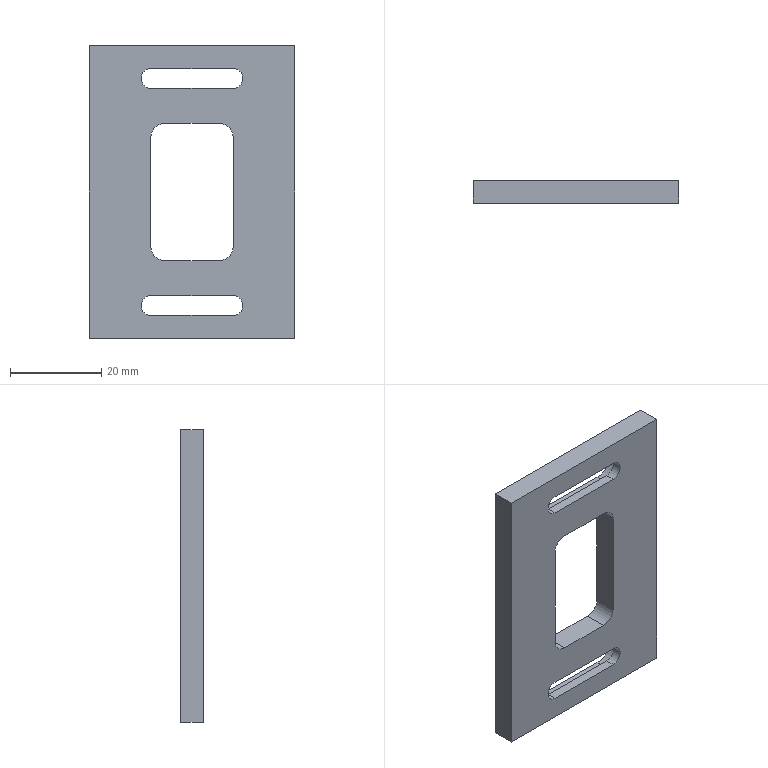Part | SolidWorks | features ICE 2, Extrusion 1, Fillet 1 | 1 solid | 32 faces | box 45 x 5 x 64 mm | volume 10150 mm3 | plane 20 | cylinder 12 | commonest cylinder face diameters 4.3 x4 6 x4 8.3 x4
STEP:
#1=CARTESIAN_POINT('',(-9.,5.,20.7));
#2=VERTEX_POINT('',#1);
#3=CARTESIAN_POINT('',(9.,5.,20.7));
#4=VERTEX_POINT('',#3);
#5=CARTESIAN_POINT('',(-9.,5.,20.7));
#6=DIRECTION('',(1.,0.,0.));
#7=VECTOR('',#6,1000.);
#8=LINE('',#5,#7);
#9=EDGE_CURVE('',#2,#4,#8,.T.);
#10=ORIENTED_EDGE('',*,*,#9,.T.);
#11=CARTESIAN_POINT('',(9.,5.,29.));
#12=VERTEX_POINT('',#11);
#13=CARTESIAN_POINT('',(9.,5.,24.85));
#14=DIRECTION('',(0.,1.,0.));
#15=DIRECTION('',(0.,0.,1.));
#16=AXIS2_PLACEMENT_3D('',#13,#14,#15);
#17=CIRCLE('',#16,4.15);
#18=EDGE_CURVE('',#12,#4,#17,.T.);
#19=ORIENTED_EDGE('',*,*,#18,.F.);
#20=CARTESIAN_POINT('',(-9.,5.,29.));
#21=VERTEX_POINT('',#20);
#22=CARTESIAN_POINT('',(-9.,5.,29.));
#23=DIRECTION('',(1.,0.,0.));
#24=VECTOR('',#23,1000.);
#25=LINE('',#22,#24);
#26=EDGE_CURVE('',#21,#12,#25,.T.);
#27=ORIENTED_EDGE('',*,*,#26,.F.);
#28=CARTESIAN_POINT('',(-9.,5.,24.85));
#29=DIRECTION('',(0.,1.,0.));
#30=DIRECTION('',(0.,0.,1.));
#31=AXIS2_PLACEMENT_3D('',#28,#29,#30);
#32=CIRCLE('',#31,4.15);
#33=EDGE_CURVE('',#2,#21,#32,.T.);
#34=ORIENTED_EDGE('',*,*,#33,.F.);
#35=EDGE_LOOP('',(#10,#19,#27,#34));
#36=FACE_BOUND('',#35,.T.);
#37=CARTESIAN_POINT('',(22.5,5.,32.));
#38=VERTEX_POINT('',#37);
#39=CARTESIAN_POINT('',(22.5,5.,-32.));
#40=VERTEX_POINT('',#39);
#41=CARTESIAN_POINT('',(22.5,5.,32.));
#42=DIRECTION('',(0.,0.,-1.));
#43=VECTOR('',#42,1000.);
#44=LINE('',#41,#43);
#45=EDGE_CURVE('',#38,#40,#44,.T.);
#46=ORIENTED_EDGE('',*,*,#45,.T.);
#47=CARTESIAN_POINT('',(-22.5,5.,-32.));
#48=VERTEX_POINT('',#47);
#49=CARTESIAN_POINT('',(-22.5,5.,-32.));
#50=DIRECTION('',(-1.,0.,0.));
#51=VECTOR('',#50,1000.);
#52=LINE('',#49,#51);
#53=EDGE_CURVE('',#40,#48,#52,.T.);
#54=ORIENTED_EDGE('',*,*,#53,.T.);
#55=CARTESIAN_POINT('',(-22.5,5.,32.));
#56=VERTEX_POINT('',#55);
#57=CARTESIAN_POINT('',(-22.5,5.,32.));
#58=DIRECTION('',(0.,0.,1.));
#59=VECTOR('',#58,1000.);
#60=LINE('',#57,#59);
#61=EDGE_CURVE('',#48,#56,#60,.T.);
#62=ORIENTED_EDGE('',*,*,#61,.T.);
#63=CARTESIAN_POINT('',(-22.5,5.,32.));
#64=DIRECTION('',(1.,0.,0.));
#65=VECTOR('',#64,1000.);
#66=LINE('',#63,#65);
#67=EDGE_CURVE('',#56,#38,#66,.T.);
#68=ORIENTED_EDGE('',*,*,#67,.T.);
#69=EDGE_LOOP('',(#46,#54,#62,#68));
#70=FACE_OUTER_BOUND('',#69,.T.);
#71=CARTESIAN_POINT('',(-9.,5.,12.));
#72=VERTEX_POINT('',#71);
#73=CARTESIAN_POINT('',(-9.,5.,-12.));
#74=VERTEX_POINT('',#73);
#75=CARTESIAN_POINT('',(-9.,5.,15.));
#76=DIRECTION('',(0.,0.,-1.));
#77=VECTOR('',#76,1000.);
#78=LINE('',#75,#77);
#79=EDGE_CURVE('',#72,#74,#78,.T.);
#80=ORIENTED_EDGE('',*,*,#79,.T.);
#81=CARTESIAN_POINT('',(-6.,5.,-15.));
#82=VERTEX_POINT('',#81);
#83=CARTESIAN_POINT('',(-6.,5.,-12.));
#84=DIRECTION('',(0.,-1.,0.));
#85=DIRECTION('',(0.,0.,-1.));
#86=AXIS2_PLACEMENT_3D('',#83,#84,#85);
#87=CIRCLE('',#86,3.);
#88=EDGE_CURVE('',#74,#82,#87,.T.);
#89=ORIENTED_EDGE('',*,*,#88,.T.);
#90=CARTESIAN_POINT('',(6.,5.,-15.));
#91=VERTEX_POINT('',#90);
#92=CARTESIAN_POINT('',(-9.,5.,-15.));
#93=DIRECTION('',(1.,0.,0.));
#94=VECTOR('',#93,1000.);
#95=LINE('',#92,#94);
#96=EDGE_CURVE('',#82,#91,#95,.T.);
#97=ORIENTED_EDGE('',*,*,#96,.T.);
#98=CARTESIAN_POINT('',(9.,5.,-12.));
#99=VERTEX_POINT('',#98);
#100=CARTESIAN_POINT('',(6.,5.,-12.));
#101=DIRECTION('',(0.,-1.,0.));
#102=DIRECTION('',(0.,0.,-1.));
#103=AXIS2_PLACEMENT_3D('',#100,#101,#102);
#104=CIRCLE('',#103,3.);
#105=EDGE_CURVE('',#91,#99,#104,.T.);
#106=ORIENTED_EDGE('',*,*,#105,.T.);
#107=CARTESIAN_POINT('',(9.,5.,12.));
#108=VERTEX_POINT('',#107);
#109=CARTESIAN_POINT('',(9.,5.,15.));
#110=DIRECTION('',(0.,0.,-1.));
#111=VECTOR('',#110,1000.);
#112=LINE('',#109,#111);
#113=EDGE_CURVE('',#108,#99,#112,.T.);
#114=ORIENTED_EDGE('',*,*,#113,.F.);
#115=CARTESIAN_POINT('',(6.,5.,15.));
#116=VERTEX_POINT('',#115);
#117=CARTESIAN_POINT('',(6.,5.,12.));
#118=DIRECTION('',(0.,-1.,0.));
#119=DIRECTION('',(0.,0.,-1.));
#120=AXIS2_PLACEMENT_3D('',#117,#118,#119);
#121=CIRCLE('',#120,3.);
#122=EDGE_CURVE('',#108,#116,#121,.T.);
#123=ORIENTED_EDGE('',*,*,#122,.T.);
#124=CARTESIAN_POINT('',(-6.,5.,15.));
#125=VERTEX_POINT('',#124);
#126=CARTESIAN_POINT('',(-9.,5.,15.));
#127=DIRECTION('',(1.,0.,0.));
#128=VECTOR('',#127,1000.);
#129=LINE('',#126,#128);
#130=EDGE_CURVE('',#125,#116,#129,.T.);
#131=ORIENTED_EDGE('',*,*,#130,.F.);
#132=CARTESIAN_POINT('',(-6.,5.,12.));
#133=DIRECTION('',(0.,-1.,0.));
#134=DIRECTION('',(0.,0.,-1.));
#135=AXIS2_PLACEMENT_3D('',#132,#133,#134);
#136=CIRCLE('',#135,3.);
#137=EDGE_CURVE('',#125,#72,#136,.T.);
#138=ORIENTED_EDGE('',*,*,#137,.T.);
#139=EDGE_LOOP('',(#80,#89,#97,#106,#114,#123,#131,#138));
#140=FACE_BOUND('',#139,.T.);
#141=CARTESIAN_POINT('',(9.,5.,-29.));
#142=VERTEX_POINT('',#141);
#143=CARTESIAN_POINT('',(9.,5.,-20.7));
#144=VERTEX_POINT('',#143);
#145=CARTESIAN_POINT('',(9.,5.,-24.85));
#146=DIRECTION('',(0.,-1.,0.));
#147=DIRECTION('',(0.,0.,-1.));
#148=AXIS2_PLACEMENT_3D('',#145,#146,#147);
#149=CIRCLE('',#148,4.15);
#150=EDGE_CURVE('',#142,#144,#149,.T.);
#151=ORIENTED_EDGE('',*,*,#150,.T.);
#152=CARTESIAN_POINT('',(-9.,5.,-20.7));
#153=VERTEX_POINT('',#152);
#154=CARTESIAN_POINT('',(-9.,5.,-20.7));
#155=DIRECTION('',(1.,0.,0.));
#156=VECTOR('',#155,1000.);
#157=LINE('',#154,#156);
#158=EDGE_CURVE('',#153,#144,#157,.T.);
#159=ORIENTED_EDGE('',*,*,#158,.F.);
#160=CARTESIAN_POINT('',(-9.,5.,-29.));
#161=VERTEX_POINT('',#160);
#162=CARTESIAN_POINT('',(-9.,5.,-24.85));
#163=DIRECTION('',(0.,-1.,0.));
#164=DIRECTION('',(0.,0.,-1.));
#165=AXIS2_PLACEMENT_3D('',#162,#163,#164);
#166=CIRCLE('',#165,4.15);
#167=EDGE_CURVE('',#153,#161,#166,.T.);
#168=ORIENTED_EDGE('',*,*,#167,.T.);
#169=CARTESIAN_POINT('',(-9.,5.,-29.));
#170=DIRECTION('',(1.,0.,0.));
#171=VECTOR('',#170,1000.);
#172=LINE('',#169,#171);
#173=EDGE_CURVE('',#161,#142,#172,.T.);
#174=ORIENTED_EDGE('',*,*,#173,.T.);
#175=EDGE_LOOP('',(#151,#159,#168,#174));
#176=FACE_BOUND('',#175,.T.);
#177=CARTESIAN_POINT('',(0.,5.,0.));
#178=DIRECTION('',(0.,-1.,0.));
#179=DIRECTION('',(0.,0.,-1.));
#180=AXIS2_PLACEMENT_3D('',#177,#178,#179);
#181=PLANE('',#180);
#182=ADVANCED_FACE('',(#36,#70,#140,#176),#181,.F.);
#183=CARTESIAN_POINT('',(-9.,2.,27.));
#184=VERTEX_POINT('',#183);
#185=CARTESIAN_POINT('',(-9.,2.,22.7));
#186=VERTEX_POINT('',#185);
#187=CARTESIAN_POINT('',(-9.,2.,24.85));
#188=DIRECTION('',(0.,-1.,0.));
#189=DIRECTION('',(0.,0.,1.));
#190=AXIS2_PLACEMENT_3D('',#187,#188,#189);
#191=CIRCLE('',#190,2.15);
#192=EDGE_CURVE('',#184,#186,#191,.T.);
#193=ORIENTED_EDGE('',*,*,#192,.F.);
#194=CARTESIAN_POINT('',(-9.,0.,27.));
#195=VERTEX_POINT('',#194);
#196=CARTESIAN_POINT('',(-9.,0.,27.));
#197=DIRECTION('',(0.,1.,0.));
#198=VECTOR('',#197,1000.);
#199=LINE('',#196,#198);
#200=EDGE_CURVE('',#195,#184,#199,.T.);
#201=ORIENTED_EDGE('',*,*,#200,.F.);
#202=CARTESIAN_POINT('',(-9.,0.,22.7));
#203=VERTEX_POINT('',#202);
#204=CARTESIAN_POINT('',(-9.,0.,24.85));
#205=DIRECTION('',(0.,1.,0.));
#206=DIRECTION('',(0.,0.,1.));
#207=AXIS2_PLACEMENT_3D('',#204,#205,#206);
#208=CIRCLE('',#207,2.15);
#209=EDGE_CURVE('',#203,#195,#208,.T.);
#210=ORIENTED_EDGE('',*,*,#209,.F.);
#211=CARTESIAN_POINT('',(-9.,0.,22.7));
#212=DIRECTION('',(0.,1.,0.));
#213=VECTOR('',#212,1000.);
#214=LINE('',#211,#213);
#215=EDGE_CURVE('',#203,#186,#214,.T.);
#216=ORIENTED_EDGE('',*,*,#215,.T.);
#217=EDGE_LOOP('',(#193,#201,#210,#216));
#218=FACE_OUTER_BOUND('',#217,.T.);
#219=CARTESIAN_POINT('',(-9.,0.,24.85));
#220=DIRECTION('',(0.,1.,0.));
#221=DIRECTION('',(0.,0.,1.));
#222=AXIS2_PLACEMENT_3D('',#219,#220,#221);
#223=CYLINDRICAL_SURFACE('',#222,2.15);
#224=ADVANCED_FACE('',(#218),#223,.F.);
#225=CARTESIAN_POINT('',(9.,0.,22.7));
#226=VERTEX_POINT('',#225);
#227=CARTESIAN_POINT('',(9.,2.,22.7));
#228=VERTEX_POINT('',#227);
#229=CARTESIAN_POINT('',(9.,0.,22.7));
#230=DIRECTION('',(0.,1.,0.));
#231=VECTOR('',#230,1000.);
#232=LINE('',#229,#231);
#233=EDGE_CURVE('',#226,#228,#232,.T.);
#234=ORIENTED_EDGE('',*,*,#233,.T.);
#235=CARTESIAN_POINT('',(-9.,2.,22.7));
#236=DIRECTION('',(-1.,0.,0.));
#237=VECTOR('',#236,1000.);
#238=LINE('',#235,#237);
#239=EDGE_CURVE('',#228,#186,#238,.T.);
#240=ORIENTED_EDGE('',*,*,#239,.T.);
#241=ORIENTED_EDGE('',*,*,#215,.F.);
#242=CARTESIAN_POINT('',(-9.,0.,22.7));
#243=DIRECTION('',(1.,0.,0.));
#244=VECTOR('',#243,1000.);
#245=LINE('',#242,#244);
#246=EDGE_CURVE('',#203,#226,#245,.T.);
#247=ORIENTED_EDGE('',*,*,#246,.T.);
#248=EDGE_LOOP('',(#234,#240,#241,#247));
#249=FACE_OUTER_BOUND('',#248,.T.);
#250=CARTESIAN_POINT('',(-9.,0.,22.7));
#251=DIRECTION('',(0.,0.,1.));
#252=DIRECTION('',(1.,0.,0.));
#253=AXIS2_PLACEMENT_3D('',#250,#251,#252);
#254=PLANE('',#253);
#255=ADVANCED_FACE('',(#249),#254,.T.);
#256=CARTESIAN_POINT('',(9.,2.,27.));
#257=VERTEX_POINT('',#256);
#258=CARTESIAN_POINT('',(9.,2.,24.85));
#259=DIRECTION('',(0.,-1.,0.));
#260=DIRECTION('',(0.,0.,1.));
#261=AXIS2_PLACEMENT_3D('',#258,#259,#260);
#262=CIRCLE('',#261,2.15);
#263=EDGE_CURVE('',#228,#257,#262,.T.);
#264=ORIENTED_EDGE('',*,*,#263,.F.);
#265=ORIENTED_EDGE('',*,*,#233,.F.);
#266=CARTESIAN_POINT('',(9.,0.,27.));
#267=VERTEX_POINT('',#266);
#268=CARTESIAN_POINT('',(9.,0.,24.85));
#269=DIRECTION('',(0.,1.,0.));
#270=DIRECTION('',(0.,0.,1.));
#271=AXIS2_PLACEMENT_3D('',#268,#269,#270);
#272=CIRCLE('',#271,2.15);
#273=EDGE_CURVE('',#267,#226,#272,.T.);
#274=ORIENTED_EDGE('',*,*,#273,.F.);
#275=CARTESIAN_POINT('',(9.,0.,27.));
#276=DIRECTION('',(0.,1.,0.));
#277=VECTOR('',#276,1000.);
#278=LINE('',#275,#277);
#279=EDGE_CURVE('',#267,#257,#278,.T.);
#280=ORIENTED_EDGE('',*,*,#279,.T.);
#281=EDGE_LOOP('',(#264,#265,#274,#280));
#282=FACE_OUTER_BOUND('',#281,.T.);
#283=CARTESIAN_POINT('',(9.,0.,24.85));
#284=DIRECTION('',(0.,1.,0.));
#285=DIRECTION('',(0.,0.,1.));
#286=AXIS2_PLACEMENT_3D('',#283,#284,#285);
#287=CYLINDRICAL_SURFACE('',#286,2.15);
#288=ADVANCED_FACE('',(#282),#287,.F.);
#289=CARTESIAN_POINT('',(-9.,2.,27.));
#290=DIRECTION('',(-1.,0.,0.));
#291=VECTOR('',#290,1000.);
#292=LINE('',#289,#291);
#293=EDGE_CURVE('',#257,#184,#292,.T.);
#294=ORIENTED_EDGE('',*,*,#293,.F.);
#295=ORIENTED_EDGE('',*,*,#279,.F.);
#296=CARTESIAN_POINT('',(-9.,0.,27.));
#297=DIRECTION('',(1.,0.,0.));
#298=VECTOR('',#297,1000.);
#299=LINE('',#296,#298);
#300=EDGE_CURVE('',#195,#267,#299,.T.);
#301=ORIENTED_EDGE('',*,*,#300,.F.);
#302=ORIENTED_EDGE('',*,*,#200,.T.);
#303=EDGE_LOOP('',(#294,#295,#301,#302));
#304=FACE_OUTER_BOUND('',#303,.T.);
#305=CARTESIAN_POINT('',(-9.,0.,27.));
#306=DIRECTION('',(0.,0.,1.));
#307=DIRECTION('',(1.,0.,0.));
#308=AXIS2_PLACEMENT_3D('',#305,#306,#307);
#309=PLANE('',#308);
#310=ADVANCED_FACE('',(#304),#309,.F.);
#311=ORIENTED_EDGE('',*,*,#209,.T.);
#312=ORIENTED_EDGE('',*,*,#300,.T.);
#313=ORIENTED_EDGE('',*,*,#273,.T.);
#314=ORIENTED_EDGE('',*,*,#246,.F.);
#315=EDGE_LOOP('',(#311,#312,#313,#314));
#316=FACE_BOUND('',#315,.T.);
#317=CARTESIAN_POINT('',(22.5,0.,32.));
#318=VERTEX_POINT('',#317);
#319=CARTESIAN_POINT('',(22.5,0.,-32.));
#320=VERTEX_POINT('',#319);
#321=CARTESIAN_POINT('',(22.5,0.,32.));
#322=DIRECTION('',(0.,0.,-1.));
#323=VECTOR('',#322,1000.);
#324=LINE('',#321,#323);
#325=EDGE_CURVE('',#318,#320,#324,.T.);
#326=ORIENTED_EDGE('',*,*,#325,.F.);
#327=CARTESIAN_POINT('',(-22.5,0.,32.));
#328=VERTEX_POINT('',#327);
#329=CARTESIAN_POINT('',(-22.5,0.,32.));
#330=DIRECTION('',(1.,0.,0.));
#331=VECTOR('',#330,1000.);
#332=LINE('',#329,#331);
#333=EDGE_CURVE('',#328,#318,#332,.T.);
#334=ORIENTED_EDGE('',*,*,#333,.F.);
#335=CARTESIAN_POINT('',(-22.5,0.,-32.));
#336=VERTEX_POINT('',#335);
#337=CARTESIAN_POINT('',(-22.5,0.,32.));
#338=DIRECTION('',(0.,0.,1.));
#339=VECTOR('',#338,1000.);
#340=LINE('',#337,#339);
#341=EDGE_CURVE('',#336,#328,#340,.T.);
#342=ORIENTED_EDGE('',*,*,#341,.F.);
#343=CARTESIAN_POINT('',(-22.5,0.,-32.));
#344=DIRECTION('',(-1.,0.,0.));
#345=VECTOR('',#344,1000.);
#346=LINE('',#343,#345);
#347=EDGE_CURVE('',#320,#336,#346,.T.);
#348=ORIENTED_EDGE('',*,*,#347,.F.);
#349=EDGE_LOOP('',(#326,#334,#342,#348));
#350=FACE_OUTER_BOUND('',#349,.T.);
#351=CARTESIAN_POINT('',(-6.,0.,15.));
#352=VERTEX_POINT('',#351);
#353=CARTESIAN_POINT('',(6.,0.,15.));
#354=VERTEX_POINT('',#353);
#355=CARTESIAN_POINT('',(-9.,0.,15.));
#356=DIRECTION('',(1.,0.,0.));
#357=VECTOR('',#356,1000.);
#358=LINE('',#355,#357);
#359=EDGE_CURVE('',#352,#354,#358,.T.);
#360=ORIENTED_EDGE('',*,*,#359,.T.);
#361=CARTESIAN_POINT('',(9.,0.,12.));
#362=VERTEX_POINT('',#361);
#363=CARTESIAN_POINT('',(6.,0.,12.));
#364=DIRECTION('',(0.,1.,0.));
#365=DIRECTION('',(0.,0.,-1.));
#366=AXIS2_PLACEMENT_3D('',#363,#364,#365);
#367=CIRCLE('',#366,3.);
#368=EDGE_CURVE('',#354,#362,#367,.T.);
#369=ORIENTED_EDGE('',*,*,#368,.T.);
#370=CARTESIAN_POINT('',(9.,0.,-12.));
#371=VERTEX_POINT('',#370);
#372=CARTESIAN_POINT('',(9.,0.,15.));
#373=DIRECTION('',(0.,0.,-1.));
#374=VECTOR('',#373,1000.);
#375=LINE('',#372,#374);
#376=EDGE_CURVE('',#362,#371,#375,.T.);
#377=ORIENTED_EDGE('',*,*,#376,.T.);
#378=CARTESIAN_POINT('',(6.,0.,-15.));
#379=VERTEX_POINT('',#378);
#380=CARTESIAN_POINT('',(6.,0.,-12.));
#381=DIRECTION('',(0.,1.,0.));
#382=DIRECTION('',(0.,0.,-1.));
#383=AXIS2_PLACEMENT_3D('',#380,#381,#382);
#384=CIRCLE('',#383,3.);
#385=EDGE_CURVE('',#371,#379,#384,.T.);
#386=ORIENTED_EDGE('',*,*,#385,.T.);
#387=CARTESIAN_POINT('',(-6.,0.,-15.));
#388=VERTEX_POINT('',#387);
#389=CARTESIAN_POINT('',(-9.,0.,-15.));
#390=DIRECTION('',(1.,0.,0.));
#391=VECTOR('',#390,1000.);
#392=LINE('',#389,#391);
#393=EDGE_CURVE('',#388,#379,#392,.T.);
#394=ORIENTED_EDGE('',*,*,#393,.F.);
#395=CARTESIAN_POINT('',(-9.,0.,-12.));
#396=VERTEX_POINT('',#395);
#397=CARTESIAN_POINT('',(-6.,0.,-12.));
#398=DIRECTION('',(0.,1.,0.));
#399=DIRECTION('',(0.,0.,-1.));
#400=AXIS2_PLACEMENT_3D('',#397,#398,#399);
#401=CIRCLE('',#400,3.);
#402=EDGE_CURVE('',#388,#396,#401,.T.);
#403=ORIENTED_EDGE('',*,*,#402,.T.);
#404=CARTESIAN_POINT('',(-9.,0.,12.));
#405=VERTEX_POINT('',#404);
#406=CARTESIAN_POINT('',(-9.,0.,15.));
#407=DIRECTION('',(0.,0.,-1.));
#408=VECTOR('',#407,1000.);
#409=LINE('',#406,#408);
#410=EDGE_CURVE('',#405,#396,#409,.T.);
#411=ORIENTED_EDGE('',*,*,#410,.F.);
#412=CARTESIAN_POINT('',(-6.,0.,12.));
#413=DIRECTION('',(0.,1.,0.));
#414=DIRECTION('',(0.,0.,-1.));
#415=AXIS2_PLACEMENT_3D('',#412,#413,#414);
#416=CIRCLE('',#415,3.);
#417=EDGE_CURVE('',#405,#352,#416,.T.);
#418=ORIENTED_EDGE('',*,*,#417,.T.);
#419=EDGE_LOOP('',(#360,#369,#377,#386,#394,#403,#411,#418));
#420=FACE_BOUND('',#419,.T.);
#421=CARTESIAN_POINT('',(-9.,0.,-27.));
#422=VERTEX_POINT('',#421);
#423=CARTESIAN_POINT('',(9.,0.,-27.));
#424=VERTEX_POINT('',#423);
#425=CARTESIAN_POINT('',(-9.,0.,-27.));
#426=DIRECTION('',(1.,0.,0.));
#427=VECTOR('',#426,1000.);
#428=LINE('',#425,#427);
#429=EDGE_CURVE('',#422,#424,#428,.T.);
#430=ORIENTED_EDGE('',*,*,#429,.F.);
#431=CARTESIAN_POINT('',(-9.,0.,-22.7));
#432=VERTEX_POINT('',#431);
#433=CARTESIAN_POINT('',(-9.,0.,-24.85));
#434=DIRECTION('',(0.,-1.,0.));
#435=DIRECTION('',(0.,0.,-1.));
#436=AXIS2_PLACEMENT_3D('',#433,#434,#435);
#437=CIRCLE('',#436,2.15);
#438=EDGE_CURVE('',#432,#422,#437,.T.);
#439=ORIENTED_EDGE('',*,*,#438,.F.);
#440=CARTESIAN_POINT('',(9.,0.,-22.7));
#441=VERTEX_POINT('',#440);
#442=CARTESIAN_POINT('',(-9.,0.,-22.7));
#443=DIRECTION('',(1.,0.,0.));
#444=VECTOR('',#443,1000.);
#445=LINE('',#442,#444);
#446=EDGE_CURVE('',#432,#441,#445,.T.);
#447=ORIENTED_EDGE('',*,*,#446,.T.);
#448=CARTESIAN_POINT('',(9.,0.,-24.85));
#449=DIRECTION('',(0.,-1.,0.));
#450=DIRECTION('',(0.,0.,-1.));
#451=AXIS2_PLACEMENT_3D('',#448,#449,#450);
#452=CIRCLE('',#451,2.15);
#453=EDGE_CURVE('',#424,#441,#452,.T.);
#454=ORIENTED_EDGE('',*,*,#453,.F.);
#455=EDGE_LOOP('',(#430,#439,#447,#454));
#456=FACE_BOUND('',#455,.T.);
#457=CARTESIAN_POINT('',(0.,0.,0.));
#458=DIRECTION('',(0.,-1.,0.));
#459=DIRECTION('',(0.,0.,-1.));
#460=AXIS2_PLACEMENT_3D('',#457,#458,#459);
#461=PLANE('',#460);
#462=ADVANCED_FACE('',(#316,#350,#420,#456),#461,.T.);
#463=ORIENTED_EDGE('',*,*,#325,.T.);
#464=CARTESIAN_POINT('',(22.5,5.,-32.));
#465=DIRECTION('',(0.,-1.,0.));
#466=VECTOR('',#465,1000.);
#467=LINE('',#464,#466);
#468=EDGE_CURVE('',#40,#320,#467,.T.);
#469=ORIENTED_EDGE('',*,*,#468,.F.);
#470=ORIENTED_EDGE('',*,*,#45,.F.);
#471=CARTESIAN_POINT('',(22.5,5.,32.));
#472=DIRECTION('',(0.,-1.,0.));
#473=VECTOR('',#472,1000.);
#474=LINE('',#471,#473);
#475=EDGE_CURVE('',#38,#318,#474,.T.);
#476=ORIENTED_EDGE('',*,*,#475,.T.);
#477=EDGE_LOOP('',(#463,#469,#470,#476));
#478=FACE_OUTER_BOUND('',#477,.T.);
#479=CARTESIAN_POINT('',(22.5,5.,32.));
#480=DIRECTION('',(-1.,0.,0.));
#481=DIRECTION('',(0.,0.,1.));
#482=AXIS2_PLACEMENT_3D('',#479,#480,#481);
#483=PLANE('',#482);
#484=ADVANCED_FACE('',(#478),#483,.F.);
#485=ORIENTED_EDGE('',*,*,#347,.T.);
#486=CARTESIAN_POINT('',(-22.5,5.,-32.));
#487=DIRECTION('',(0.,-1.,0.));
#488=VECTOR('',#487,1000.);
#489=LINE('',#486,#488);
#490=EDGE_CURVE('',#48,#336,#489,.T.);
#491=ORIENTED_EDGE('',*,*,#490,.F.);
#492=ORIENTED_EDGE('',*,*,#53,.F.);
#493=ORIENTED_EDGE('',*,*,#468,.T.);
#494=EDGE_LOOP('',(#485,#491,#492,#493));
#495=FACE_OUTER_BOUND('',#494,.T.);
#496=CARTESIAN_POINT('',(-22.5,5.,-32.));
#497=DIRECTION('',(0.,0.,1.));
#498=DIRECTION('',(1.,0.,0.));
#499=AXIS2_PLACEMENT_3D('',#496,#497,#498);
#500=PLANE('',#499);
#501=ADVANCED_FACE('',(#495),#500,.F.);
#502=ORIENTED_EDGE('',*,*,#341,.T.);
#503=CARTESIAN_POINT('',(-22.5,5.,32.));
#504=DIRECTION('',(0.,-1.,0.));
#505=VECTOR('',#504,1000.);
#506=LINE('',#503,#505);
#507=EDGE_CURVE('',#56,#328,#506,.T.);
#508=ORIENTED_EDGE('',*,*,#507,.F.);
#509=ORIENTED_EDGE('',*,*,#61,.F.);
#510=ORIENTED_EDGE('',*,*,#490,.T.);
#511=EDGE_LOOP('',(#502,#508,#509,#510));
#512=FACE_OUTER_BOUND('',#511,.T.);
#513=CARTESIAN_POINT('',(-22.5,5.,32.));
#514=DIRECTION('',(1.,0.,0.));
#515=DIRECTION('',(0.,0.,-1.));
#516=AXIS2_PLACEMENT_3D('',#513,#514,#515);
#517=PLANE('',#516);
#518=ADVANCED_FACE('',(#512),#517,.F.);
#519=ORIENTED_EDGE('',*,*,#333,.T.);
#520=ORIENTED_EDGE('',*,*,#475,.F.);
#521=ORIENTED_EDGE('',*,*,#67,.F.);
#522=ORIENTED_EDGE('',*,*,#507,.T.);
#523=EDGE_LOOP('',(#519,#520,#521,#522));
#524=FACE_OUTER_BOUND('',#523,.T.);
#525=CARTESIAN_POINT('',(-22.5,5.,32.));
#526=DIRECTION('',(0.,0.,-1.));
#527=DIRECTION('',(-1.,0.,0.));
#528=AXIS2_PLACEMENT_3D('',#525,#526,#527);
#529=PLANE('',#528);
#530=ADVANCED_FACE('',(#524),#529,.F.);
#531=ORIENTED_EDGE('',*,*,#393,.T.);
#532=CARTESIAN_POINT('',(6.,0.,-15.));
#533=DIRECTION('',(0.,1.,0.));
#534=VECTOR('',#533,1000.);
#535=LINE('',#532,#534);
#536=EDGE_CURVE('',#379,#91,#535,.T.);
#537=ORIENTED_EDGE('',*,*,#536,.T.);
#538=ORIENTED_EDGE('',*,*,#96,.F.);
#539=CARTESIAN_POINT('',(-6.,0.,-15.));
#540=DIRECTION('',(0.,-1.,0.));
#541=VECTOR('',#540,1000.);
#542=LINE('',#539,#541);
#543=EDGE_CURVE('',#82,#388,#542,.T.);
#544=ORIENTED_EDGE('',*,*,#543,.T.);
#545=EDGE_LOOP('',(#531,#537,#538,#544));
#546=FACE_OUTER_BOUND('',#545,.T.);
#547=CARTESIAN_POINT('',(-9.,0.,-15.));
#548=DIRECTION('',(0.,0.,1.));
#549=DIRECTION('',(1.,0.,0.));
#550=AXIS2_PLACEMENT_3D('',#547,#548,#549);
#551=PLANE('',#550);
#552=ADVANCED_FACE('',(#546),#551,.T.);
#553=ORIENTED_EDGE('',*,*,#113,.T.);
#554=CARTESIAN_POINT('',(9.,0.,-12.));
#555=DIRECTION('',(0.,-1.,0.));
#556=VECTOR('',#555,1000.);
#557=LINE('',#554,#556);
#558=EDGE_CURVE('',#99,#371,#557,.T.);
#559=ORIENTED_EDGE('',*,*,#558,.T.);
#560=ORIENTED_EDGE('',*,*,#376,.F.);
#561=CARTESIAN_POINT('',(9.,5.,12.));
#562=DIRECTION('',(0.,1.,0.));
#563=VECTOR('',#562,1000.);
#564=LINE('',#561,#563);
#565=EDGE_CURVE('',#362,#108,#564,.T.);
#566=ORIENTED_EDGE('',*,*,#565,.T.);
#567=EDGE_LOOP('',(#553,#559,#560,#566));
#568=FACE_OUTER_BOUND('',#567,.T.);
#569=CARTESIAN_POINT('',(9.,0.,15.));
#570=DIRECTION('',(1.,0.,0.));
#571=DIRECTION('',(0.,0.,-1.));
#572=AXIS2_PLACEMENT_3D('',#569,#570,#571);
#573=PLANE('',#572);
#574=ADVANCED_FACE('',(#568),#573,.F.);
#575=ORIENTED_EDGE('',*,*,#130,.T.);
#576=CARTESIAN_POINT('',(6.,0.,15.));
#577=DIRECTION('',(0.,-1.,0.));
#578=VECTOR('',#577,1000.);
#579=LINE('',#576,#578);
#580=EDGE_CURVE('',#116,#354,#579,.T.);
#581=ORIENTED_EDGE('',*,*,#580,.T.);
#582=ORIENTED_EDGE('',*,*,#359,.F.);
#583=CARTESIAN_POINT('',(-6.,0.,15.));
#584=DIRECTION('',(0.,1.,0.));
#585=VECTOR('',#584,1000.);
#586=LINE('',#583,#585);
#587=EDGE_CURVE('',#352,#125,#586,.T.);
#588=ORIENTED_EDGE('',*,*,#587,.T.);
#589=EDGE_LOOP('',(#575,#581,#582,#588));
#590=FACE_OUTER_BOUND('',#589,.T.);
#591=CARTESIAN_POINT('',(-9.,0.,15.));
#592=DIRECTION('',(0.,0.,1.));
#593=DIRECTION('',(1.,0.,0.));
#594=AXIS2_PLACEMENT_3D('',#591,#592,#593);
#595=PLANE('',#594);
#596=ADVANCED_FACE('',(#590),#595,.F.);
#597=ORIENTED_EDGE('',*,*,#79,.F.);
#598=CARTESIAN_POINT('',(-9.,0.,12.));
#599=DIRECTION('',(0.,-1.,0.));
#600=VECTOR('',#599,1000.);
#601=LINE('',#598,#600);
#602=EDGE_CURVE('',#72,#405,#601,.T.);
#603=ORIENTED_EDGE('',*,*,#602,.T.);
#604=ORIENTED_EDGE('',*,*,#410,.T.);
#605=CARTESIAN_POINT('',(-9.,5.,-12.));
#606=DIRECTION('',(0.,1.,0.));
#607=VECTOR('',#606,1000.);
#608=LINE('',#605,#607);
#609=EDGE_CURVE('',#396,#74,#608,.T.);
#610=ORIENTED_EDGE('',*,*,#609,.T.);
#611=EDGE_LOOP('',(#597,#603,#604,#610));
#612=FACE_OUTER_BOUND('',#611,.T.);
#613=CARTESIAN_POINT('',(-9.,0.,15.));
#614=DIRECTION('',(1.,0.,0.));
#615=DIRECTION('',(0.,0.,-1.));
#616=AXIS2_PLACEMENT_3D('',#613,#614,#615);
#617=PLANE('',#616);
#618=ADVANCED_FACE('',(#612),#617,.T.);
#619=CARTESIAN_POINT('',(-9.,2.,-22.7));
#620=VERTEX_POINT('',#619);
#621=CARTESIAN_POINT('',(-9.,2.,-27.));
#622=VERTEX_POINT('',#621);
#623=CARTESIAN_POINT('',(-9.,2.,-24.85));
#624=DIRECTION('',(0.,-1.,0.));
#625=DIRECTION('',(0.,0.,-1.));
#626=AXIS2_PLACEMENT_3D('',#623,#624,#625);
#627=CIRCLE('',#626,2.15);
#628=EDGE_CURVE('',#620,#622,#627,.T.);
#629=ORIENTED_EDGE('',*,*,#628,.F.);
#630=CARTESIAN_POINT('',(-9.,0.,-22.7));
#631=DIRECTION('',(0.,1.,0.));
#632=VECTOR('',#631,1000.);
#633=LINE('',#630,#632);
#634=EDGE_CURVE('',#432,#620,#633,.T.);
#635=ORIENTED_EDGE('',*,*,#634,.F.);
#636=ORIENTED_EDGE('',*,*,#438,.T.);
#637=CARTESIAN_POINT('',(-9.,0.,-27.));
#638=DIRECTION('',(0.,1.,0.));
#639=VECTOR('',#638,1000.);
#640=LINE('',#637,#639);
#641=EDGE_CURVE('',#422,#622,#640,.T.);
#642=ORIENTED_EDGE('',*,*,#641,.T.);
#643=EDGE_LOOP('',(#629,#635,#636,#642));
#644=FACE_OUTER_BOUND('',#643,.T.);
#645=CARTESIAN_POINT('',(-9.,0.,-24.85));
#646=DIRECTION('',(0.,1.,0.));
#647=DIRECTION('',(0.,0.,1.));
#648=AXIS2_PLACEMENT_3D('',#645,#646,#647);
#649=CYLINDRICAL_SURFACE('',#648,2.15);
#650=ADVANCED_FACE('',(#644),#649,.F.);
#651=CARTESIAN_POINT('',(9.,2.,-27.));
#652=VERTEX_POINT('',#651);
#653=CARTESIAN_POINT('',(-9.,2.,-27.));
#654=DIRECTION('',(1.,0.,0.));
#655=VECTOR('',#654,1000.);
#656=LINE('',#653,#655);
#657=EDGE_CURVE('',#622,#652,#656,.T.);
#658=ORIENTED_EDGE('',*,*,#657,.F.);
#659=ORIENTED_EDGE('',*,*,#641,.F.);
#660=ORIENTED_EDGE('',*,*,#429,.T.);
#661=CARTESIAN_POINT('',(9.,0.,-27.));
#662=DIRECTION('',(0.,1.,0.));
#663=VECTOR('',#662,1000.);
#664=LINE('',#661,#663);
#665=EDGE_CURVE('',#424,#652,#664,.T.);
#666=ORIENTED_EDGE('',*,*,#665,.T.);
#667=EDGE_LOOP('',(#658,#659,#660,#666));
#668=FACE_OUTER_BOUND('',#667,.T.);
#669=CARTESIAN_POINT('',(-9.,0.,-27.));
#670=DIRECTION('',(0.,0.,1.));
#671=DIRECTION('',(1.,0.,0.));
#672=AXIS2_PLACEMENT_3D('',#669,#670,#671);
#673=PLANE('',#672);
#674=ADVANCED_FACE('',(#668),#673,.T.);
#675=CARTESIAN_POINT('',(9.,2.,-22.7));
#676=VERTEX_POINT('',#675);
#677=CARTESIAN_POINT('',(9.,2.,-24.85));
#678=DIRECTION('',(0.,-1.,0.));
#679=DIRECTION('',(0.,0.,-1.));
#680=AXIS2_PLACEMENT_3D('',#677,#678,#679);
#681=CIRCLE('',#680,2.15);
#682=EDGE_CURVE('',#652,#676,#681,.T.);
#683=ORIENTED_EDGE('',*,*,#682,.F.);
#684=ORIENTED_EDGE('',*,*,#665,.F.);
#685=ORIENTED_EDGE('',*,*,#453,.T.);
#686=CARTESIAN_POINT('',(9.,0.,-22.7));
#687=DIRECTION('',(0.,1.,0.));
#688=VECTOR('',#687,1000.);
#689=LINE('',#686,#688);
#690=EDGE_CURVE('',#441,#676,#689,.T.);
#691=ORIENTED_EDGE('',*,*,#690,.T.);
#692=EDGE_LOOP('',(#683,#684,#685,#691));
#693=FACE_OUTER_BOUND('',#692,.T.);
#694=CARTESIAN_POINT('',(9.,0.,-24.85));
#695=DIRECTION('',(0.,1.,0.));
#696=DIRECTION('',(0.,0.,1.));
#697=AXIS2_PLACEMENT_3D('',#694,#695,#696);
#698=CYLINDRICAL_SURFACE('',#697,2.15);
#699=ADVANCED_FACE('',(#693),#698,.F.);
#700=ORIENTED_EDGE('',*,*,#634,.T.);
#701=CARTESIAN_POINT('',(-9.,2.,-22.7));
#702=DIRECTION('',(1.,0.,0.));
#703=VECTOR('',#702,1000.);
#704=LINE('',#701,#703);
#705=EDGE_CURVE('',#620,#676,#704,.T.);
#706=ORIENTED_EDGE('',*,*,#705,.T.);
#707=ORIENTED_EDGE('',*,*,#690,.F.);
#708=ORIENTED_EDGE('',*,*,#446,.F.);
#709=EDGE_LOOP('',(#700,#706,#707,#708));
#710=FACE_OUTER_BOUND('',#709,.T.);
#711=CARTESIAN_POINT('',(-9.,0.,-22.7));
#712=DIRECTION('',(0.,0.,1.));
#713=DIRECTION('',(1.,0.,0.));
#714=AXIS2_PLACEMENT_3D('',#711,#712,#713);
#715=PLANE('',#714);
#716=ADVANCED_FACE('',(#710),#715,.F.);
#717=ORIENTED_EDGE('',*,*,#158,.T.);
#718=CARTESIAN_POINT('',(9.,2.,-20.7));
#719=VERTEX_POINT('',#718);
#720=CARTESIAN_POINT('',(9.,2.,-20.7));
#721=DIRECTION('',(0.,1.,0.));
#722=VECTOR('',#721,1000.);
#723=LINE('',#720,#722);
#724=EDGE_CURVE('',#719,#144,#723,.T.);
#725=ORIENTED_EDGE('',*,*,#724,.F.);
#726=CARTESIAN_POINT('',(-9.,2.,-20.7));
#727=VERTEX_POINT('',#726);
#728=CARTESIAN_POINT('',(-9.,2.,-20.7));
#729=DIRECTION('',(1.,0.,0.));
#730=VECTOR('',#729,1000.);
#731=LINE('',#728,#730);
#732=EDGE_CURVE('',#727,#719,#731,.T.);
#733=ORIENTED_EDGE('',*,*,#732,.F.);
#734=CARTESIAN_POINT('',(-9.,2.,-20.7));
#735=DIRECTION('',(0.,1.,0.));
#736=VECTOR('',#735,1000.);
#737=LINE('',#734,#736);
#738=EDGE_CURVE('',#727,#153,#737,.T.);
#739=ORIENTED_EDGE('',*,*,#738,.T.);
#740=EDGE_LOOP('',(#717,#725,#733,#739));
#741=FACE_OUTER_BOUND('',#740,.T.);
#742=CARTESIAN_POINT('',(-9.,2.,-20.7));
#743=DIRECTION('',(0.,0.,1.));
#744=DIRECTION('',(1.,0.,0.));
#745=AXIS2_PLACEMENT_3D('',#742,#743,#744);
#746=PLANE('',#745);
#747=ADVANCED_FACE('',(#741),#746,.F.);
#748=ORIENTED_EDGE('',*,*,#167,.F.);
#749=ORIENTED_EDGE('',*,*,#738,.F.);
#750=CARTESIAN_POINT('',(-9.,2.,-29.));
#751=VERTEX_POINT('',#750);
#752=CARTESIAN_POINT('',(-9.,2.,-24.85));
#753=DIRECTION('',(0.,-1.,0.));
#754=DIRECTION('',(0.,0.,-1.));
#755=AXIS2_PLACEMENT_3D('',#752,#753,#754);
#756=CIRCLE('',#755,4.15);
#757=EDGE_CURVE('',#727,#751,#756,.T.);
#758=ORIENTED_EDGE('',*,*,#757,.T.);
#759=CARTESIAN_POINT('',(-9.,2.,-29.));
#760=DIRECTION('',(0.,1.,0.));
#761=VECTOR('',#760,1000.);
#762=LINE('',#759,#761);
#763=EDGE_CURVE('',#751,#161,#762,.T.);
#764=ORIENTED_EDGE('',*,*,#763,.T.);
#765=EDGE_LOOP('',(#748,#749,#758,#764));
#766=FACE_OUTER_BOUND('',#765,.T.);
#767=CARTESIAN_POINT('',(-9.,2.,-24.85));
#768=DIRECTION('',(0.,1.,0.));
#769=DIRECTION('',(0.,0.,1.));
#770=AXIS2_PLACEMENT_3D('',#767,#768,#769);
#771=CYLINDRICAL_SURFACE('',#770,4.15);
#772=ADVANCED_FACE('',(#766),#771,.F.);
#773=ORIENTED_EDGE('',*,*,#173,.F.);
#774=ORIENTED_EDGE('',*,*,#763,.F.);
#775=CARTESIAN_POINT('',(9.,2.,-29.));
#776=VERTEX_POINT('',#775);
#777=CARTESIAN_POINT('',(-9.,2.,-29.));
#778=DIRECTION('',(1.,0.,0.));
#779=VECTOR('',#778,1000.);
#780=LINE('',#777,#779);
#781=EDGE_CURVE('',#751,#776,#780,.T.);
#782=ORIENTED_EDGE('',*,*,#781,.T.);
#783=CARTESIAN_POINT('',(9.,2.,-29.));
#784=DIRECTION('',(0.,1.,0.));
#785=VECTOR('',#784,1000.);
#786=LINE('',#783,#785);
#787=EDGE_CURVE('',#776,#142,#786,.T.);
#788=ORIENTED_EDGE('',*,*,#787,.T.);
#789=EDGE_LOOP('',(#773,#774,#782,#788));
#790=FACE_OUTER_BOUND('',#789,.T.);
#791=CARTESIAN_POINT('',(-9.,2.,-29.));
#792=DIRECTION('',(0.,0.,1.));
#793=DIRECTION('',(1.,0.,0.));
#794=AXIS2_PLACEMENT_3D('',#791,#792,#793);
#795=PLANE('',#794);
#796=ADVANCED_FACE('',(#790),#795,.T.);
#797=ORIENTED_EDGE('',*,*,#150,.F.);
#798=ORIENTED_EDGE('',*,*,#787,.F.);
#799=CARTESIAN_POINT('',(9.,2.,-24.85));
#800=DIRECTION('',(0.,-1.,0.));
#801=DIRECTION('',(0.,0.,-1.));
#802=AXIS2_PLACEMENT_3D('',#799,#800,#801);
#803=CIRCLE('',#802,4.15);
#804=EDGE_CURVE('',#776,#719,#803,.T.);
#805=ORIENTED_EDGE('',*,*,#804,.T.);
#806=ORIENTED_EDGE('',*,*,#724,.T.);
#807=EDGE_LOOP('',(#797,#798,#805,#806));
#808=FACE_OUTER_BOUND('',#807,.T.);
#809=CARTESIAN_POINT('',(9.,2.,-24.85));
#810=DIRECTION('',(0.,1.,0.));
#811=DIRECTION('',(0.,0.,1.));
#812=AXIS2_PLACEMENT_3D('',#809,#810,#811);
#813=CYLINDRICAL_SURFACE('',#812,4.15);
#814=ADVANCED_FACE('',(#808),#813,.F.);
#815=ORIENTED_EDGE('',*,*,#628,.T.);
#816=ORIENTED_EDGE('',*,*,#657,.T.);
#817=ORIENTED_EDGE('',*,*,#682,.T.);
#818=ORIENTED_EDGE('',*,*,#705,.F.);
#819=EDGE_LOOP('',(#815,#816,#817,#818));
#820=FACE_BOUND('',#819,.T.);
#821=ORIENTED_EDGE('',*,*,#732,.T.);
#822=ORIENTED_EDGE('',*,*,#804,.F.);
#823=ORIENTED_EDGE('',*,*,#781,.F.);
#824=ORIENTED_EDGE('',*,*,#757,.F.);
#825=EDGE_LOOP('',(#821,#822,#823,#824));
#826=FACE_OUTER_BOUND('',#825,.T.);
#827=CARTESIAN_POINT('',(9.,2.,-24.85));
#828=DIRECTION('',(0.,-1.,0.));
#829=DIRECTION('',(0.,0.,-1.));
#830=AXIS2_PLACEMENT_3D('',#827,#828,#829);
#831=PLANE('',#830);
#832=ADVANCED_FACE('',(#820,#826),#831,.F.);
#833=CARTESIAN_POINT('',(-9.,2.,20.7));
#834=VERTEX_POINT('',#833);
#835=CARTESIAN_POINT('',(9.,2.,20.7));
#836=VERTEX_POINT('',#835);
#837=CARTESIAN_POINT('',(-9.,2.,20.7));
#838=DIRECTION('',(1.,0.,0.));
#839=VECTOR('',#838,1000.);
#840=LINE('',#837,#839);
#841=EDGE_CURVE('',#834,#836,#840,.T.);
#842=ORIENTED_EDGE('',*,*,#841,.F.);
#843=CARTESIAN_POINT('',(-9.,2.,29.));
#844=VERTEX_POINT('',#843);
#845=CARTESIAN_POINT('',(-9.,2.,24.85));
#846=DIRECTION('',(0.,1.,0.));
#847=DIRECTION('',(0.,0.,1.));
#848=AXIS2_PLACEMENT_3D('',#845,#846,#847);
#849=CIRCLE('',#848,4.15);
#850=EDGE_CURVE('',#834,#844,#849,.T.);
#851=ORIENTED_EDGE('',*,*,#850,.T.);
#852=CARTESIAN_POINT('',(9.,2.,29.));
#853=VERTEX_POINT('',#852);
#854=CARTESIAN_POINT('',(-9.,2.,29.));
#855=DIRECTION('',(1.,0.,0.));
#856=VECTOR('',#855,1000.);
#857=LINE('',#854,#856);
#858=EDGE_CURVE('',#844,#853,#857,.T.);
#859=ORIENTED_EDGE('',*,*,#858,.T.);
#860=CARTESIAN_POINT('',(9.,2.,24.85));
#861=DIRECTION('',(0.,1.,0.));
#862=DIRECTION('',(0.,0.,1.));
#863=AXIS2_PLACEMENT_3D('',#860,#861,#862);
#864=CIRCLE('',#863,4.15);
#865=EDGE_CURVE('',#853,#836,#864,.T.);
#866=ORIENTED_EDGE('',*,*,#865,.T.);
#867=EDGE_LOOP('',(#842,#851,#859,#866));
#868=FACE_OUTER_BOUND('',#867,.T.);
#869=ORIENTED_EDGE('',*,*,#192,.T.);
#870=ORIENTED_EDGE('',*,*,#239,.F.);
#871=ORIENTED_EDGE('',*,*,#263,.T.);
#872=ORIENTED_EDGE('',*,*,#293,.T.);
#873=EDGE_LOOP('',(#869,#870,#871,#872));
#874=FACE_BOUND('',#873,.T.);
#875=CARTESIAN_POINT('',(9.,2.,24.85));
#876=DIRECTION('',(0.,1.,0.));
#877=DIRECTION('',(0.,0.,1.));
#878=AXIS2_PLACEMENT_3D('',#875,#876,#877);
#879=PLANE('',#878);
#880=ADVANCED_FACE('',(#868,#874),#879,.T.);
#881=ORIENTED_EDGE('',*,*,#9,.F.);
#882=CARTESIAN_POINT('',(-9.,2.,20.7));
#883=DIRECTION('',(0.,1.,0.));
#884=VECTOR('',#883,1000.);
#885=LINE('',#882,#884);
#886=EDGE_CURVE('',#834,#2,#885,.T.);
#887=ORIENTED_EDGE('',*,*,#886,.F.);
#888=ORIENTED_EDGE('',*,*,#841,.T.);
#889=CARTESIAN_POINT('',(9.,2.,20.7));
#890=DIRECTION('',(0.,1.,0.));
#891=VECTOR('',#890,1000.);
#892=LINE('',#889,#891);
#893=EDGE_CURVE('',#836,#4,#892,.T.);
#894=ORIENTED_EDGE('',*,*,#893,.T.);
#895=EDGE_LOOP('',(#881,#887,#888,#894));
#896=FACE_OUTER_BOUND('',#895,.T.);
#897=CARTESIAN_POINT('',(-9.,2.,20.7));
#898=DIRECTION('',(0.,0.,1.));
#899=DIRECTION('',(1.,0.,0.));
#900=AXIS2_PLACEMENT_3D('',#897,#898,#899);
#901=PLANE('',#900);
#902=ADVANCED_FACE('',(#896),#901,.T.);
#903=ORIENTED_EDGE('',*,*,#18,.T.);
#904=ORIENTED_EDGE('',*,*,#893,.F.);
#905=ORIENTED_EDGE('',*,*,#865,.F.);
#906=CARTESIAN_POINT('',(9.,2.,29.));
#907=DIRECTION('',(0.,1.,0.));
#908=VECTOR('',#907,1000.);
#909=LINE('',#906,#908);
#910=EDGE_CURVE('',#853,#12,#909,.T.);
#911=ORIENTED_EDGE('',*,*,#910,.T.);
#912=EDGE_LOOP('',(#903,#904,#905,#911));
#913=FACE_OUTER_BOUND('',#912,.T.);
#914=CARTESIAN_POINT('',(9.,2.,24.85));
#915=DIRECTION('',(0.,1.,0.));
#916=DIRECTION('',(0.,0.,1.));
#917=AXIS2_PLACEMENT_3D('',#914,#915,#916);
#918=CYLINDRICAL_SURFACE('',#917,4.15);
#919=ADVANCED_FACE('',(#913),#918,.F.);
#920=ORIENTED_EDGE('',*,*,#26,.T.);
#921=ORIENTED_EDGE('',*,*,#910,.F.);
#922=ORIENTED_EDGE('',*,*,#858,.F.);
#923=CARTESIAN_POINT('',(-9.,2.,29.));
#924=DIRECTION('',(0.,1.,0.));
#925=VECTOR('',#924,1000.);
#926=LINE('',#923,#925);
#927=EDGE_CURVE('',#844,#21,#926,.T.);
#928=ORIENTED_EDGE('',*,*,#927,.T.);
#929=EDGE_LOOP('',(#920,#921,#922,#928));
#930=FACE_OUTER_BOUND('',#929,.T.);
#931=CARTESIAN_POINT('',(-9.,2.,29.));
#932=DIRECTION('',(0.,0.,1.));
#933=DIRECTION('',(1.,0.,0.));
#934=AXIS2_PLACEMENT_3D('',#931,#932,#933);
#935=PLANE('',#934);
#936=ADVANCED_FACE('',(#930),#935,.F.);
#937=ORIENTED_EDGE('',*,*,#33,.T.);
#938=ORIENTED_EDGE('',*,*,#927,.F.);
#939=ORIENTED_EDGE('',*,*,#850,.F.);
#940=ORIENTED_EDGE('',*,*,#886,.T.);
#941=EDGE_LOOP('',(#937,#938,#939,#940));
#942=FACE_OUTER_BOUND('',#941,.T.);
#943=CARTESIAN_POINT('',(-9.,2.,24.85));
#944=DIRECTION('',(0.,1.,0.));
#945=DIRECTION('',(0.,0.,1.));
#946=AXIS2_PLACEMENT_3D('',#943,#944,#945);
#947=CYLINDRICAL_SURFACE('',#946,4.15);
#948=ADVANCED_FACE('',(#942),#947,.F.);
#949=ORIENTED_EDGE('',*,*,#385,.F.);
#950=ORIENTED_EDGE('',*,*,#558,.F.);
#951=ORIENTED_EDGE('',*,*,#105,.F.);
#952=ORIENTED_EDGE('',*,*,#536,.F.);
#953=EDGE_LOOP('',(#949,#950,#951,#952));
#954=FACE_OUTER_BOUND('',#953,.T.);
#955=CARTESIAN_POINT('',(6.,0.,-12.));
#956=DIRECTION('',(0.,1.,0.));
#957=DIRECTION('',(0.,0.,1.));
#958=AXIS2_PLACEMENT_3D('',#955,#956,#957);
#959=CYLINDRICAL_SURFACE('',#958,3.);
#960=ADVANCED_FACE('',(#954),#959,.F.);
#961=ORIENTED_EDGE('',*,*,#368,.F.);
#962=ORIENTED_EDGE('',*,*,#580,.F.);
#963=ORIENTED_EDGE('',*,*,#122,.F.);
#964=ORIENTED_EDGE('',*,*,#565,.F.);
#965=EDGE_LOOP('',(#961,#962,#963,#964));
#966=FACE_OUTER_BOUND('',#965,.T.);
#967=CARTESIAN_POINT('',(6.,0.,12.));
#968=DIRECTION('',(0.,-1.,0.));
#969=DIRECTION('',(0.,0.,-1.));
#970=AXIS2_PLACEMENT_3D('',#967,#968,#969);
#971=CYLINDRICAL_SURFACE('',#970,3.);
#972=ADVANCED_FACE('',(#966),#971,.F.);
#973=ORIENTED_EDGE('',*,*,#417,.F.);
#974=ORIENTED_EDGE('',*,*,#602,.F.);
#975=ORIENTED_EDGE('',*,*,#137,.F.);
#976=ORIENTED_EDGE('',*,*,#587,.F.);
#977=EDGE_LOOP('',(#973,#974,#975,#976));
#978=FACE_OUTER_BOUND('',#977,.T.);
#979=CARTESIAN_POINT('',(-6.,0.,12.));
#980=DIRECTION('',(0.,1.,0.));
#981=DIRECTION('',(0.,0.,1.));
#982=AXIS2_PLACEMENT_3D('',#979,#980,#981);
#983=CYLINDRICAL_SURFACE('',#982,3.);
#984=ADVANCED_FACE('',(#978),#983,.F.);
#985=ORIENTED_EDGE('',*,*,#402,.F.);
#986=ORIENTED_EDGE('',*,*,#543,.F.);
#987=ORIENTED_EDGE('',*,*,#88,.F.);
#988=ORIENTED_EDGE('',*,*,#609,.F.);
#989=EDGE_LOOP('',(#985,#986,#987,#988));
#990=FACE_OUTER_BOUND('',#989,.T.);
#991=CARTESIAN_POINT('',(-6.,0.,-12.));
#992=DIRECTION('',(0.,-1.,0.));
#993=DIRECTION('',(0.,0.,-1.));
#994=AXIS2_PLACEMENT_3D('',#991,#992,#993);
#995=CYLINDRICAL_SURFACE('',#994,3.);
#996=ADVANCED_FACE('',(#990),#995,.F.);
#997=CLOSED_SHELL('',(#182,#224,#255,#288,#310,#462,#484,#501,#518,#530,#552,#574,#596,#618,#650,#674,#699,#716,#747,#772,#796,#814,#832,#880,#902,#919,#936,#948,#960,#972,#984,#996));
#998=MANIFOLD_SOLID_BREP('',#997);
#999=CARTESIAN_POINT('',(0.,0.,0.));
#1000=DIRECTION('',(0.,0.,1.));
#1001=DIRECTION('',(1.,0.,0.));
#1002=AXIS2_PLACEMENT_3D('',#999,#1000,#1001);
#1003=(LENGTH_UNIT()NAMED_UNIT(*)SI_UNIT(.MILLI.,.METRE.));
#1004=UNCERTAINTY_MEASURE_WITH_UNIT(LENGTH_MEASURE(0.00001),#1003,'','');
#1005=(NAMED_UNIT(*)PLANE_ANGLE_UNIT()SI_UNIT($,.RADIAN.));
#1006=(NAMED_UNIT(*)SI_UNIT($,.STERADIAN.)SOLID_ANGLE_UNIT());
#1007=(GEOMETRIC_REPRESENTATION_CONTEXT(3)GLOBAL_UNCERTAINTY_ASSIGNED_CONTEXT((#1004))GLOBAL_UNIT_ASSIGNED_CONTEXT((#1003,#1005,#1006))REPRESENTATION_CONTEXT('',''));
#1008=ADVANCED_BREP_SHAPE_REPRESENTATION('',(#998,#1002),#1007);